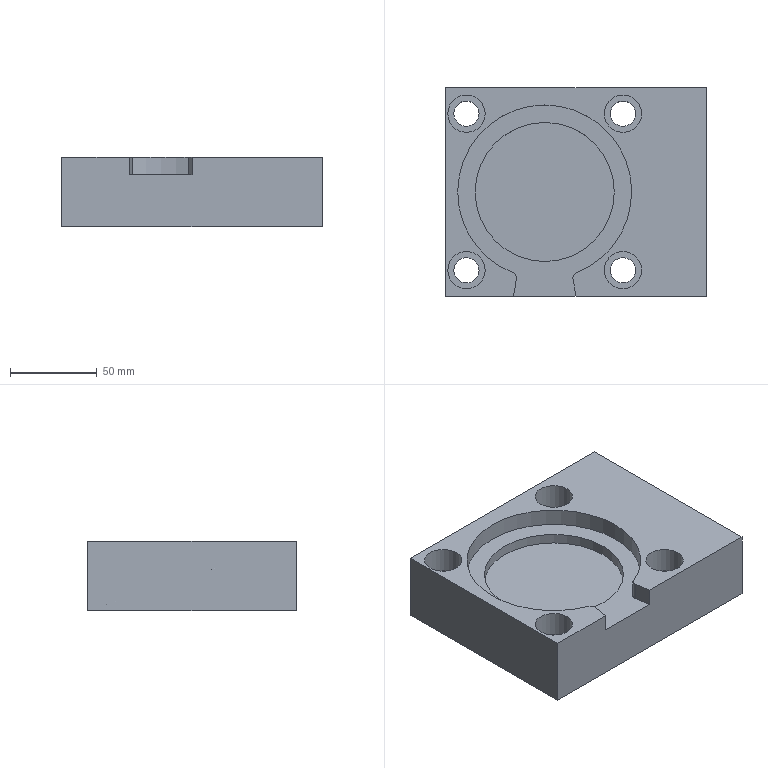Part | NX | 1 solid | 26 faces | box 150 x 120 x 40 mm | volume 569278 mm3 | plane 14 | cylinder 12 | commonest cylinder face diameters 14.5 x4 21.5 x4 6 x2 80 x1 100 x1
STEP:
#1=CARTESIAN_POINT('',(0.,-60.,-10.));
#2=VERTEX_POINT('',#1);
#3=CARTESIAN_POINT('',(-36.,-60.,-10.));
#4=VERTEX_POINT('',#3);
#5=CARTESIAN_POINT('',(0.,-60.,-10.));
#6=DIRECTION('',(-1.,0.,0.));
#7=VECTOR('',#6,1000.);
#8=LINE('',#5,#7);
#9=EDGE_CURVE('',#2,#4,#8,.T.);
#10=ORIENTED_EDGE('',*,*,#9,.T.);
#11=CARTESIAN_POINT('',(-36.,-60.,0.));
#12=VERTEX_POINT('',#11);
#13=CARTESIAN_POINT('',(-36.,-60.,-10.));
#14=DIRECTION('',(0.,0.,1.));
#15=VECTOR('',#14,1000.);
#16=LINE('',#13,#15);
#17=EDGE_CURVE('',#4,#12,#16,.T.);
#18=ORIENTED_EDGE('',*,*,#17,.T.);
#19=CARTESIAN_POINT('',(-75.,-60.,0.));
#20=VERTEX_POINT('',#19);
#21=CARTESIAN_POINT('',(-75.,-60.,0.));
#22=DIRECTION('',(1.,0.,0.));
#23=VECTOR('',#22,1000.);
#24=LINE('',#21,#23);
#25=EDGE_CURVE('',#20,#12,#24,.T.);
#26=ORIENTED_EDGE('',*,*,#25,.F.);
#27=CARTESIAN_POINT('',(-75.,-60.,-40.));
#28=VERTEX_POINT('',#27);
#29=CARTESIAN_POINT('',(-75.,-60.,-40.));
#30=DIRECTION('',(0.,0.,1.));
#31=VECTOR('',#30,1000.);
#32=LINE('',#29,#31);
#33=EDGE_CURVE('',#28,#20,#32,.T.);
#34=ORIENTED_EDGE('',*,*,#33,.F.);
#35=CARTESIAN_POINT('',(75.,-60.,-40.));
#36=VERTEX_POINT('',#35);
#37=CARTESIAN_POINT('',(-75.,-60.,-40.));
#38=DIRECTION('',(1.,0.,0.));
#39=VECTOR('',#38,1000.);
#40=LINE('',#37,#39);
#41=EDGE_CURVE('',#28,#36,#40,.T.);
#42=ORIENTED_EDGE('',*,*,#41,.T.);
#43=CARTESIAN_POINT('',(75.,-60.,0.));
#44=VERTEX_POINT('',#43);
#45=CARTESIAN_POINT('',(75.,-60.,-40.));
#46=DIRECTION('',(0.,0.,1.));
#47=VECTOR('',#46,1000.);
#48=LINE('',#45,#47);
#49=EDGE_CURVE('',#36,#44,#48,.T.);
#50=ORIENTED_EDGE('',*,*,#49,.T.);
#51=CARTESIAN_POINT('',(0.,-60.,0.));
#52=VERTEX_POINT('',#51);
#53=CARTESIAN_POINT('',(-75.,-60.,0.));
#54=DIRECTION('',(1.,0.,0.));
#55=VECTOR('',#54,1000.);
#56=LINE('',#53,#55);
#57=EDGE_CURVE('',#52,#44,#56,.T.);
#58=ORIENTED_EDGE('',*,*,#57,.F.);
#59=CARTESIAN_POINT('',(0.,-60.,-10.));
#60=DIRECTION('',(0.,0.,1.));
#61=VECTOR('',#60,1000.);
#62=LINE('',#59,#61);
#63=EDGE_CURVE('',#2,#52,#62,.T.);
#64=ORIENTED_EDGE('',*,*,#63,.F.);
#65=EDGE_LOOP('',(#10,#18,#26,#34,#42,#50,#58,#64));
#66=FACE_BOUND('',#65,.T.);
#67=CARTESIAN_POINT('',(-75.,-60.,-40.));
#68=DIRECTION('',(0.,-1.,0.));
#69=DIRECTION('',(0.,0.,-1.));
#70=AXIS2_PLACEMENT_3D('',#67,#68,#69);
#71=PLANE('',#70);
#72=ADVANCED_FACE('',(#66),#71,.T.);
#73=CARTESIAN_POINT('',(34.25,-45.,-40.));
#74=VERTEX_POINT('',#73);
#75=CARTESIAN_POINT('',(27.,-45.,-40.));
#76=DIRECTION('',(0.,0.,1.));
#77=DIRECTION('',(1.,0.,0.));
#78=AXIS2_PLACEMENT_3D('',#75,#76,#77);
#79=CIRCLE('',#78,7.25);
#80=EDGE_CURVE('',#74,#74,#79,.T.);
#81=ORIENTED_EDGE('',*,*,#80,.F.);
#82=EDGE_LOOP('',(#81));
#83=FACE_BOUND('',#82,.T.);
#84=CARTESIAN_POINT('',(34.25,-45.,-15.));
#85=VERTEX_POINT('',#84);
#86=CARTESIAN_POINT('',(27.,-45.,-15.));
#87=DIRECTION('',(0.,0.,1.));
#88=DIRECTION('',(1.,0.,0.));
#89=AXIS2_PLACEMENT_3D('',#86,#87,#88);
#90=CIRCLE('',#89,7.25);
#91=EDGE_CURVE('',#85,#85,#90,.F.);
#92=ORIENTED_EDGE('',*,*,#91,.F.);
#93=EDGE_LOOP('',(#92));
#94=FACE_BOUND('',#93,.T.);
#95=CARTESIAN_POINT('',(27.,-45.,-40.));
#96=DIRECTION('',(0.,0.,1.));
#97=DIRECTION('',(1.,0.,0.));
#98=AXIS2_PLACEMENT_3D('',#95,#96,#97);
#99=CYLINDRICAL_SURFACE('',#98,7.25);
#100=ADVANCED_FACE('',(#83,#94),#99,.F.);
#101=CARTESIAN_POINT('',(-55.75,45.,-40.));
#102=VERTEX_POINT('',#101);
#103=CARTESIAN_POINT('',(-63.,45.,-40.));
#104=DIRECTION('',(0.,0.,1.));
#105=DIRECTION('',(1.,0.,0.));
#106=AXIS2_PLACEMENT_3D('',#103,#104,#105);
#107=CIRCLE('',#106,7.25);
#108=EDGE_CURVE('',#102,#102,#107,.T.);
#109=ORIENTED_EDGE('',*,*,#108,.F.);
#110=EDGE_LOOP('',(#109));
#111=FACE_BOUND('',#110,.T.);
#112=CARTESIAN_POINT('',(-55.75,45.,-15.));
#113=VERTEX_POINT('',#112);
#114=CARTESIAN_POINT('',(-63.,45.,-15.));
#115=DIRECTION('',(0.,0.,1.));
#116=DIRECTION('',(1.,0.,0.));
#117=AXIS2_PLACEMENT_3D('',#114,#115,#116);
#118=CIRCLE('',#117,7.25);
#119=EDGE_CURVE('',#113,#113,#118,.F.);
#120=ORIENTED_EDGE('',*,*,#119,.F.);
#121=EDGE_LOOP('',(#120));
#122=FACE_BOUND('',#121,.T.);
#123=CARTESIAN_POINT('',(-63.,45.,-40.));
#124=DIRECTION('',(0.,0.,1.));
#125=DIRECTION('',(1.,0.,0.));
#126=AXIS2_PLACEMENT_3D('',#123,#124,#125);
#127=CYLINDRICAL_SURFACE('',#126,7.25);
#128=ADVANCED_FACE('',(#111,#122),#127,.F.);
#129=CARTESIAN_POINT('',(-55.75,-45.,-40.));
#130=VERTEX_POINT('',#129);
#131=CARTESIAN_POINT('',(-63.,-45.,-40.));
#132=DIRECTION('',(0.,0.,1.));
#133=DIRECTION('',(1.,0.,0.));
#134=AXIS2_PLACEMENT_3D('',#131,#132,#133);
#135=CIRCLE('',#134,7.25);
#136=EDGE_CURVE('',#130,#130,#135,.T.);
#137=ORIENTED_EDGE('',*,*,#136,.F.);
#138=EDGE_LOOP('',(#137));
#139=FACE_BOUND('',#138,.T.);
#140=CARTESIAN_POINT('',(-55.75,-45.,-15.));
#141=VERTEX_POINT('',#140);
#142=CARTESIAN_POINT('',(-63.,-45.,-15.));
#143=DIRECTION('',(0.,0.,1.));
#144=DIRECTION('',(1.,0.,0.));
#145=AXIS2_PLACEMENT_3D('',#142,#143,#144);
#146=CIRCLE('',#145,7.25);
#147=EDGE_CURVE('',#141,#141,#146,.F.);
#148=ORIENTED_EDGE('',*,*,#147,.F.);
#149=EDGE_LOOP('',(#148));
#150=FACE_BOUND('',#149,.T.);
#151=CARTESIAN_POINT('',(-63.,-45.,-40.));
#152=DIRECTION('',(0.,0.,1.));
#153=DIRECTION('',(1.,0.,0.));
#154=AXIS2_PLACEMENT_3D('',#151,#152,#153);
#155=CYLINDRICAL_SURFACE('',#154,7.25);
#156=ADVANCED_FACE('',(#139,#150),#155,.F.);
#157=CARTESIAN_POINT('',(34.25,45.,-40.));
#158=VERTEX_POINT('',#157);
#159=CARTESIAN_POINT('',(27.,45.,-40.));
#160=DIRECTION('',(0.,0.,1.));
#161=DIRECTION('',(1.,0.,0.));
#162=AXIS2_PLACEMENT_3D('',#159,#160,#161);
#163=CIRCLE('',#162,7.25);
#164=EDGE_CURVE('',#158,#158,#163,.T.);
#165=ORIENTED_EDGE('',*,*,#164,.F.);
#166=EDGE_LOOP('',(#165));
#167=FACE_BOUND('',#166,.T.);
#168=CARTESIAN_POINT('',(34.25,45.,-15.));
#169=VERTEX_POINT('',#168);
#170=CARTESIAN_POINT('',(27.,45.,-15.));
#171=DIRECTION('',(0.,0.,1.));
#172=DIRECTION('',(1.,0.,0.));
#173=AXIS2_PLACEMENT_3D('',#170,#171,#172);
#174=CIRCLE('',#173,7.25);
#175=EDGE_CURVE('',#169,#169,#174,.F.);
#176=ORIENTED_EDGE('',*,*,#175,.F.);
#177=EDGE_LOOP('',(#176));
#178=FACE_BOUND('',#177,.T.);
#179=CARTESIAN_POINT('',(27.,45.,-40.));
#180=DIRECTION('',(0.,0.,1.));
#181=DIRECTION('',(1.,0.,0.));
#182=AXIS2_PLACEMENT_3D('',#179,#180,#181);
#183=CYLINDRICAL_SURFACE('',#182,7.25);
#184=ADVANCED_FACE('',(#167,#178),#183,.F.);
#185=CARTESIAN_POINT('',(75.,60.,0.));
#186=VERTEX_POINT('',#185);
#187=CARTESIAN_POINT('',(75.,-60.,0.));
#188=DIRECTION('',(0.,1.,0.));
#189=VECTOR('',#188,1000.);
#190=LINE('',#187,#189);
#191=EDGE_CURVE('',#44,#186,#190,.T.);
#192=ORIENTED_EDGE('',*,*,#191,.F.);
#193=ORIENTED_EDGE('',*,*,#49,.F.);
#194=CARTESIAN_POINT('',(75.,60.,-40.));
#195=VERTEX_POINT('',#194);
#196=CARTESIAN_POINT('',(75.,-60.,-40.));
#197=DIRECTION('',(0.,1.,0.));
#198=VECTOR('',#197,1000.);
#199=LINE('',#196,#198);
#200=EDGE_CURVE('',#36,#195,#199,.T.);
#201=ORIENTED_EDGE('',*,*,#200,.T.);
#202=CARTESIAN_POINT('',(75.,60.,-40.));
#203=DIRECTION('',(0.,0.,1.));
#204=VECTOR('',#203,1000.);
#205=LINE('',#202,#204);
#206=EDGE_CURVE('',#195,#186,#205,.T.);
#207=ORIENTED_EDGE('',*,*,#206,.T.);
#208=EDGE_LOOP('',(#192,#193,#201,#207));
#209=FACE_BOUND('',#208,.T.);
#210=CARTESIAN_POINT('',(75.,-60.,-40.));
#211=DIRECTION('',(1.,0.,0.));
#212=DIRECTION('',(0.,1.,0.));
#213=AXIS2_PLACEMENT_3D('',#210,#211,#212);
#214=PLANE('',#213);
#215=ADVANCED_FACE('',(#209),#214,.T.);
#216=CARTESIAN_POINT('',(-75.,60.,0.));
#217=VERTEX_POINT('',#216);
#218=CARTESIAN_POINT('',(75.,60.,0.));
#219=DIRECTION('',(-1.,0.,0.));
#220=VECTOR('',#219,1000.);
#221=LINE('',#218,#220);
#222=EDGE_CURVE('',#186,#217,#221,.T.);
#223=ORIENTED_EDGE('',*,*,#222,.F.);
#224=ORIENTED_EDGE('',*,*,#206,.F.);
#225=CARTESIAN_POINT('',(-75.,60.,-40.));
#226=VERTEX_POINT('',#225);
#227=CARTESIAN_POINT('',(75.,60.,-40.));
#228=DIRECTION('',(-1.,0.,0.));
#229=VECTOR('',#228,1000.);
#230=LINE('',#227,#229);
#231=EDGE_CURVE('',#195,#226,#230,.T.);
#232=ORIENTED_EDGE('',*,*,#231,.T.);
#233=CARTESIAN_POINT('',(-75.,60.,-40.));
#234=DIRECTION('',(0.,0.,1.));
#235=VECTOR('',#234,1000.);
#236=LINE('',#233,#235);
#237=EDGE_CURVE('',#226,#217,#236,.T.);
#238=ORIENTED_EDGE('',*,*,#237,.T.);
#239=EDGE_LOOP('',(#223,#224,#232,#238));
#240=FACE_BOUND('',#239,.T.);
#241=CARTESIAN_POINT('',(75.,60.,-40.));
#242=DIRECTION('',(0.,1.,0.));
#243=DIRECTION('',(-1.,0.,0.));
#244=AXIS2_PLACEMENT_3D('',#241,#242,#243);
#245=PLANE('',#244);
#246=ADVANCED_FACE('',(#240),#245,.T.);
#247=CARTESIAN_POINT('',(-75.,60.,0.));
#248=DIRECTION('',(0.,-1.,0.));
#249=VECTOR('',#248,1000.);
#250=LINE('',#247,#249);
#251=EDGE_CURVE('',#217,#20,#250,.T.);
#252=ORIENTED_EDGE('',*,*,#251,.F.);
#253=ORIENTED_EDGE('',*,*,#237,.F.);
#254=CARTESIAN_POINT('',(-75.,60.,-40.));
#255=DIRECTION('',(0.,-1.,0.));
#256=VECTOR('',#255,1000.);
#257=LINE('',#254,#256);
#258=EDGE_CURVE('',#226,#28,#257,.T.);
#259=ORIENTED_EDGE('',*,*,#258,.T.);
#260=ORIENTED_EDGE('',*,*,#33,.T.);
#261=EDGE_LOOP('',(#252,#253,#259,#260));
#262=FACE_BOUND('',#261,.T.);
#263=CARTESIAN_POINT('',(-75.,60.,-40.));
#264=DIRECTION('',(-1.,0.,0.));
#265=DIRECTION('',(0.,-1.,0.));
#266=AXIS2_PLACEMENT_3D('',#263,#264,#265);
#267=PLANE('',#266);
#268=ADVANCED_FACE('',(#262),#267,.T.);
#269=ORIENTED_EDGE('',*,*,#41,.F.);
#270=ORIENTED_EDGE('',*,*,#258,.F.);
#271=ORIENTED_EDGE('',*,*,#231,.F.);
#272=ORIENTED_EDGE('',*,*,#200,.F.);
#273=EDGE_LOOP('',(#269,#270,#271,#272));
#274=FACE_BOUND('',#273,.T.);
#275=ORIENTED_EDGE('',*,*,#136,.T.);
#276=EDGE_LOOP('',(#275));
#277=FACE_BOUND('',#276,.T.);
#278=ORIENTED_EDGE('',*,*,#108,.T.);
#279=EDGE_LOOP('',(#278));
#280=FACE_BOUND('',#279,.T.);
#281=ORIENTED_EDGE('',*,*,#80,.T.);
#282=EDGE_LOOP('',(#281));
#283=FACE_BOUND('',#282,.T.);
#284=ORIENTED_EDGE('',*,*,#164,.T.);
#285=EDGE_LOOP('',(#284));
#286=FACE_BOUND('',#285,.T.);
#287=CARTESIAN_POINT('',(-63.,-45.,-40.));
#288=DIRECTION('',(0.,0.,1.));
#289=DIRECTION('',(1.,0.,0.));
#290=AXIS2_PLACEMENT_3D('',#287,#288,#289);
#291=PLANE('',#290);
#292=ADVANCED_FACE('',(#274,#277,#280,#283,#286),#291,.F.);
#293=CARTESIAN_POINT('',(37.75,-45.,0.));
#294=VERTEX_POINT('',#293);
#295=CARTESIAN_POINT('',(27.,-45.,0.));
#296=DIRECTION('',(0.,0.,1.));
#297=DIRECTION('',(1.,0.,0.));
#298=AXIS2_PLACEMENT_3D('',#295,#296,#297);
#299=CIRCLE('',#298,10.75);
#300=EDGE_CURVE('',#294,#294,#299,.T.);
#301=ORIENTED_EDGE('',*,*,#300,.F.);
#302=EDGE_LOOP('',(#301));
#303=FACE_BOUND('',#302,.T.);
#304=CARTESIAN_POINT('',(-52.25,45.,0.));
#305=VERTEX_POINT('',#304);
#306=CARTESIAN_POINT('',(-63.,45.,0.));
#307=DIRECTION('',(0.,0.,1.));
#308=DIRECTION('',(1.,0.,0.));
#309=AXIS2_PLACEMENT_3D('',#306,#307,#308);
#310=CIRCLE('',#309,10.75);
#311=EDGE_CURVE('',#305,#305,#310,.T.);
#312=ORIENTED_EDGE('',*,*,#311,.F.);
#313=EDGE_LOOP('',(#312));
#314=FACE_BOUND('',#313,.T.);
#315=CARTESIAN_POINT('',(-52.25,-45.,0.));
#316=VERTEX_POINT('',#315);
#317=CARTESIAN_POINT('',(-63.,-45.,0.));
#318=DIRECTION('',(0.,0.,1.));
#319=DIRECTION('',(1.,0.,0.));
#320=AXIS2_PLACEMENT_3D('',#317,#318,#319);
#321=CIRCLE('',#320,10.75);
#322=EDGE_CURVE('',#316,#316,#321,.T.);
#323=ORIENTED_EDGE('',*,*,#322,.F.);
#324=EDGE_LOOP('',(#323));
#325=FACE_BOUND('',#324,.T.);
#326=CARTESIAN_POINT('',(37.75,45.,0.));
#327=VERTEX_POINT('',#326);
#328=CARTESIAN_POINT('',(27.,45.,0.));
#329=DIRECTION('',(0.,0.,1.));
#330=DIRECTION('',(1.,0.,0.));
#331=AXIS2_PLACEMENT_3D('',#328,#329,#330);
#332=CIRCLE('',#331,10.75);
#333=EDGE_CURVE('',#327,#327,#332,.T.);
#334=ORIENTED_EDGE('',*,*,#333,.F.);
#335=EDGE_LOOP('',(#334));
#336=FACE_BOUND('',#335,.T.);
#337=CARTESIAN_POINT('',(-36.093,-46.612,0.));
#338=VERTEX_POINT('',#337);
#339=CARTESIAN_POINT('',(0.09309,-46.612,0.));
#340=VERTEX_POINT('',#339);
#341=CARTESIAN_POINT('',(-18.,0.,0.));
#342=DIRECTION('',(0.,0.,-1.));
#343=DIRECTION('',(1.,0.,0.));
#344=AXIS2_PLACEMENT_3D('',#341,#342,#343);
#345=CIRCLE('',#344,50.);
#346=EDGE_CURVE('',#338,#340,#345,.T.);
#347=ORIENTED_EDGE('',*,*,#346,.T.);
#348=CARTESIAN_POINT('',(-1.776,-49.929,0.));
#349=VERTEX_POINT('',#348);
#350=CARTESIAN_POINT('',(1.179,-49.408,0.));
#351=DIRECTION('',(0.,0.,1.));
#352=DIRECTION('',(1.,0.,0.));
#353=AXIS2_PLACEMENT_3D('',#350,#351,#352);
#354=CIRCLE('',#353,3.);
#355=EDGE_CURVE('',#340,#349,#354,.T.);
#356=ORIENTED_EDGE('',*,*,#355,.T.);
#357=CARTESIAN_POINT('',(-2.214,-47.443,0.));
#358=DIRECTION('',(0.1736,-0.9848,0.));
#359=VECTOR('',#358,1000.);
#360=LINE('',#357,#359);
#361=EDGE_CURVE('',#349,#52,#360,.T.);
#362=ORIENTED_EDGE('',*,*,#361,.T.);
#363=ORIENTED_EDGE('',*,*,#57,.T.);
#364=ORIENTED_EDGE('',*,*,#191,.T.);
#365=ORIENTED_EDGE('',*,*,#222,.T.);
#366=ORIENTED_EDGE('',*,*,#251,.T.);
#367=ORIENTED_EDGE('',*,*,#25,.T.);
#368=CARTESIAN_POINT('',(-34.224,-49.929,0.));
#369=VERTEX_POINT('',#368);
#370=CARTESIAN_POINT('',(-36.,-60.,0.));
#371=DIRECTION('',(0.1736,0.9848,0.));
#372=VECTOR('',#371,1000.);
#373=LINE('',#370,#372);
#374=EDGE_CURVE('',#12,#369,#373,.T.);
#375=ORIENTED_EDGE('',*,*,#374,.T.);
#376=CARTESIAN_POINT('',(-37.179,-49.408,0.));
#377=DIRECTION('',(0.,0.,1.));
#378=DIRECTION('',(1.,0.,0.));
#379=AXIS2_PLACEMENT_3D('',#376,#377,#378);
#380=CIRCLE('',#379,3.);
#381=EDGE_CURVE('',#369,#338,#380,.T.);
#382=ORIENTED_EDGE('',*,*,#381,.T.);
#383=EDGE_LOOP('',(#347,#356,#362,#363,#364,#365,#366,#367,#375,#382));
#384=FACE_BOUND('',#383,.T.);
#385=CARTESIAN_POINT('',(-63.,-45.,0.));
#386=DIRECTION('',(0.,0.,1.));
#387=DIRECTION('',(1.,0.,0.));
#388=AXIS2_PLACEMENT_3D('',#385,#386,#387);
#389=PLANE('',#388);
#390=ADVANCED_FACE('',(#303,#314,#325,#336,#384),#389,.T.);
#391=CARTESIAN_POINT('',(37.75,45.,-15.));
#392=VERTEX_POINT('',#391);
#393=CARTESIAN_POINT('',(27.,45.,-15.));
#394=DIRECTION('',(0.,0.,1.));
#395=DIRECTION('',(1.,0.,0.));
#396=AXIS2_PLACEMENT_3D('',#393,#394,#395);
#397=CIRCLE('',#396,10.75);
#398=EDGE_CURVE('',#392,#392,#397,.F.);
#399=ORIENTED_EDGE('',*,*,#398,.F.);
#400=EDGE_LOOP('',(#399));
#401=FACE_BOUND('',#400,.T.);
#402=ORIENTED_EDGE('',*,*,#175,.T.);
#403=EDGE_LOOP('',(#402));
#404=FACE_BOUND('',#403,.T.);
#405=CARTESIAN_POINT('',(27.,45.,-15.));
#406=DIRECTION('',(0.,0.,1.));
#407=DIRECTION('',(1.,0.,0.));
#408=AXIS2_PLACEMENT_3D('',#405,#406,#407);
#409=PLANE('',#408);
#410=ADVANCED_FACE('',(#401,#404),#409,.T.);
#411=ORIENTED_EDGE('',*,*,#398,.T.);
#412=EDGE_LOOP('',(#411));
#413=FACE_BOUND('',#412,.T.);
#414=ORIENTED_EDGE('',*,*,#333,.T.);
#415=EDGE_LOOP('',(#414));
#416=FACE_BOUND('',#415,.T.);
#417=CARTESIAN_POINT('',(27.,45.,-15.));
#418=DIRECTION('',(0.,0.,1.));
#419=DIRECTION('',(1.,0.,0.));
#420=AXIS2_PLACEMENT_3D('',#417,#418,#419);
#421=CYLINDRICAL_SURFACE('',#420,10.75);
#422=ADVANCED_FACE('',(#413,#416),#421,.F.);
#423=CARTESIAN_POINT('',(-52.25,-45.,-15.));
#424=VERTEX_POINT('',#423);
#425=CARTESIAN_POINT('',(-63.,-45.,-15.));
#426=DIRECTION('',(0.,0.,1.));
#427=DIRECTION('',(1.,0.,0.));
#428=AXIS2_PLACEMENT_3D('',#425,#426,#427);
#429=CIRCLE('',#428,10.75);
#430=EDGE_CURVE('',#424,#424,#429,.F.);
#431=ORIENTED_EDGE('',*,*,#430,.F.);
#432=EDGE_LOOP('',(#431));
#433=FACE_BOUND('',#432,.T.);
#434=ORIENTED_EDGE('',*,*,#147,.T.);
#435=EDGE_LOOP('',(#434));
#436=FACE_BOUND('',#435,.T.);
#437=CARTESIAN_POINT('',(-63.,-45.,-15.));
#438=DIRECTION('',(0.,0.,1.));
#439=DIRECTION('',(1.,0.,0.));
#440=AXIS2_PLACEMENT_3D('',#437,#438,#439);
#441=PLANE('',#440);
#442=ADVANCED_FACE('',(#433,#436),#441,.T.);
#443=ORIENTED_EDGE('',*,*,#430,.T.);
#444=EDGE_LOOP('',(#443));
#445=FACE_BOUND('',#444,.T.);
#446=ORIENTED_EDGE('',*,*,#322,.T.);
#447=EDGE_LOOP('',(#446));
#448=FACE_BOUND('',#447,.T.);
#449=CARTESIAN_POINT('',(-63.,-45.,-15.));
#450=DIRECTION('',(0.,0.,1.));
#451=DIRECTION('',(1.,0.,0.));
#452=AXIS2_PLACEMENT_3D('',#449,#450,#451);
#453=CYLINDRICAL_SURFACE('',#452,10.75);
#454=ADVANCED_FACE('',(#445,#448),#453,.F.);
#455=CARTESIAN_POINT('',(-52.25,45.,-15.));
#456=VERTEX_POINT('',#455);
#457=CARTESIAN_POINT('',(-63.,45.,-15.));
#458=DIRECTION('',(0.,0.,1.));
#459=DIRECTION('',(1.,0.,0.));
#460=AXIS2_PLACEMENT_3D('',#457,#458,#459);
#461=CIRCLE('',#460,10.75);
#462=EDGE_CURVE('',#456,#456,#461,.F.);
#463=ORIENTED_EDGE('',*,*,#462,.F.);
#464=EDGE_LOOP('',(#463));
#465=FACE_BOUND('',#464,.T.);
#466=ORIENTED_EDGE('',*,*,#119,.T.);
#467=EDGE_LOOP('',(#466));
#468=FACE_BOUND('',#467,.T.);
#469=CARTESIAN_POINT('',(-63.,45.,-15.));
#470=DIRECTION('',(0.,0.,1.));
#471=DIRECTION('',(1.,0.,0.));
#472=AXIS2_PLACEMENT_3D('',#469,#470,#471);
#473=PLANE('',#472);
#474=ADVANCED_FACE('',(#465,#468),#473,.T.);
#475=ORIENTED_EDGE('',*,*,#462,.T.);
#476=EDGE_LOOP('',(#475));
#477=FACE_BOUND('',#476,.T.);
#478=ORIENTED_EDGE('',*,*,#311,.T.);
#479=EDGE_LOOP('',(#478));
#480=FACE_BOUND('',#479,.T.);
#481=CARTESIAN_POINT('',(-63.,45.,-15.));
#482=DIRECTION('',(0.,0.,1.));
#483=DIRECTION('',(1.,0.,0.));
#484=AXIS2_PLACEMENT_3D('',#481,#482,#483);
#485=CYLINDRICAL_SURFACE('',#484,10.75);
#486=ADVANCED_FACE('',(#477,#480),#485,.F.);
#487=CARTESIAN_POINT('',(37.75,-45.,-15.));
#488=VERTEX_POINT('',#487);
#489=CARTESIAN_POINT('',(27.,-45.,-15.));
#490=DIRECTION('',(0.,0.,1.));
#491=DIRECTION('',(1.,0.,0.));
#492=AXIS2_PLACEMENT_3D('',#489,#490,#491);
#493=CIRCLE('',#492,10.75);
#494=EDGE_CURVE('',#488,#488,#493,.F.);
#495=ORIENTED_EDGE('',*,*,#494,.F.);
#496=EDGE_LOOP('',(#495));
#497=FACE_BOUND('',#496,.T.);
#498=ORIENTED_EDGE('',*,*,#91,.T.);
#499=EDGE_LOOP('',(#498));
#500=FACE_BOUND('',#499,.T.);
#501=CARTESIAN_POINT('',(27.,-45.,-15.));
#502=DIRECTION('',(0.,0.,1.));
#503=DIRECTION('',(1.,0.,0.));
#504=AXIS2_PLACEMENT_3D('',#501,#502,#503);
#505=PLANE('',#504);
#506=ADVANCED_FACE('',(#497,#500),#505,.T.);
#507=ORIENTED_EDGE('',*,*,#494,.T.);
#508=EDGE_LOOP('',(#507));
#509=FACE_BOUND('',#508,.T.);
#510=ORIENTED_EDGE('',*,*,#300,.T.);
#511=EDGE_LOOP('',(#510));
#512=FACE_BOUND('',#511,.T.);
#513=CARTESIAN_POINT('',(27.,-45.,-15.));
#514=DIRECTION('',(0.,0.,1.));
#515=DIRECTION('',(1.,0.,0.));
#516=AXIS2_PLACEMENT_3D('',#513,#514,#515);
#517=CYLINDRICAL_SURFACE('',#516,10.75);
#518=ADVANCED_FACE('',(#509,#512),#517,.F.);
#519=ORIENTED_EDGE('',*,*,#9,.F.);
#520=CARTESIAN_POINT('',(-1.776,-49.929,-10.));
#521=VERTEX_POINT('',#520);
#522=CARTESIAN_POINT('',(-2.214,-47.443,-10.));
#523=DIRECTION('',(0.1736,-0.9848,0.));
#524=VECTOR('',#523,1000.);
#525=LINE('',#522,#524);
#526=EDGE_CURVE('',#2,#521,#525,.F.);
#527=ORIENTED_EDGE('',*,*,#526,.T.);
#528=CARTESIAN_POINT('',(0.09309,-46.612,-10.));
#529=VERTEX_POINT('',#528);
#530=CARTESIAN_POINT('',(1.179,-49.408,-10.));
#531=DIRECTION('',(0.,0.,-1.));
#532=DIRECTION('',(-1.,0.,0.));
#533=AXIS2_PLACEMENT_3D('',#530,#531,#532);
#534=CIRCLE('',#533,3.);
#535=EDGE_CURVE('',#521,#529,#534,.T.);
#536=ORIENTED_EDGE('',*,*,#535,.T.);
#537=CARTESIAN_POINT('',(-36.093,-46.612,-10.));
#538=VERTEX_POINT('',#537);
#539=CARTESIAN_POINT('',(-18.,0.,-10.));
#540=DIRECTION('',(0.,0.,-1.));
#541=DIRECTION('',(1.,0.,0.));
#542=AXIS2_PLACEMENT_3D('',#539,#540,#541);
#543=CIRCLE('',#542,50.);
#544=EDGE_CURVE('',#529,#538,#543,.F.);
#545=ORIENTED_EDGE('',*,*,#544,.T.);
#546=CARTESIAN_POINT('',(-34.224,-49.929,-10.));
#547=VERTEX_POINT('',#546);
#548=CARTESIAN_POINT('',(-37.179,-49.408,-10.));
#549=DIRECTION('',(0.,0.,-1.));
#550=DIRECTION('',(-1.,0.,0.));
#551=AXIS2_PLACEMENT_3D('',#548,#549,#550);
#552=CIRCLE('',#551,3.);
#553=EDGE_CURVE('',#538,#547,#552,.T.);
#554=ORIENTED_EDGE('',*,*,#553,.T.);
#555=CARTESIAN_POINT('',(-36.,-60.,-10.));
#556=DIRECTION('',(0.1736,0.9848,0.));
#557=VECTOR('',#556,1000.);
#558=LINE('',#555,#557);
#559=EDGE_CURVE('',#547,#4,#558,.F.);
#560=ORIENTED_EDGE('',*,*,#559,.T.);
#561=EDGE_LOOP('',(#519,#527,#536,#545,#554,#560));
#562=FACE_BOUND('',#561,.T.);
#563=CARTESIAN_POINT('',(-58.,0.,-10.));
#564=VERTEX_POINT('',#563);
#565=CARTESIAN_POINT('',(-18.,0.,-10.));
#566=DIRECTION('',(0.,0.,-1.));
#567=DIRECTION('',(-1.,0.,0.));
#568=AXIS2_PLACEMENT_3D('',#565,#566,#567);
#569=CIRCLE('',#568,40.);
#570=EDGE_CURVE('',#564,#564,#569,.F.);
#571=ORIENTED_EDGE('',*,*,#570,.F.);
#572=EDGE_LOOP('',(#571));
#573=FACE_BOUND('',#572,.T.);
#574=CARTESIAN_POINT('',(-18.,0.,-10.));
#575=DIRECTION('',(0.,0.,-1.));
#576=DIRECTION('',(-1.,0.,0.));
#577=AXIS2_PLACEMENT_3D('',#574,#575,#576);
#578=PLANE('',#577);
#579=ADVANCED_FACE('',(#562,#573),#578,.F.);
#580=ORIENTED_EDGE('',*,*,#559,.F.);
#581=CARTESIAN_POINT('',(-34.224,-49.929,-10.));
#582=DIRECTION('',(0.,0.,1.));
#583=VECTOR('',#582,1000.);
#584=LINE('',#581,#583);
#585=EDGE_CURVE('',#547,#369,#584,.T.);
#586=ORIENTED_EDGE('',*,*,#585,.T.);
#587=ORIENTED_EDGE('',*,*,#374,.F.);
#588=ORIENTED_EDGE('',*,*,#17,.F.);
#589=EDGE_LOOP('',(#580,#586,#587,#588));
#590=FACE_BOUND('',#589,.T.);
#591=CARTESIAN_POINT('',(-36.,-60.,-10.));
#592=DIRECTION('',(0.9848,-0.1736,0.));
#593=DIRECTION('',(0.1736,0.9848,0.));
#594=AXIS2_PLACEMENT_3D('',#591,#592,#593);
#595=PLANE('',#594);
#596=ADVANCED_FACE('',(#590),#595,.T.);
#597=ORIENTED_EDGE('',*,*,#544,.F.);
#598=CARTESIAN_POINT('',(0.09309,-46.612,-10.));
#599=DIRECTION('',(0.,0.,1.));
#600=VECTOR('',#599,1000.);
#601=LINE('',#598,#600);
#602=EDGE_CURVE('',#529,#340,#601,.T.);
#603=ORIENTED_EDGE('',*,*,#602,.T.);
#604=ORIENTED_EDGE('',*,*,#346,.F.);
#605=CARTESIAN_POINT('',(-36.093,-46.612,-10.));
#606=DIRECTION('',(0.,0.,1.));
#607=VECTOR('',#606,1000.);
#608=LINE('',#605,#607);
#609=EDGE_CURVE('',#338,#538,#608,.F.);
#610=ORIENTED_EDGE('',*,*,#609,.T.);
#611=EDGE_LOOP('',(#597,#603,#604,#610));
#612=FACE_BOUND('',#611,.T.);
#613=CARTESIAN_POINT('',(-18.,0.,-10.));
#614=DIRECTION('',(0.,0.,1.));
#615=DIRECTION('',(1.,0.,0.));
#616=AXIS2_PLACEMENT_3D('',#613,#614,#615);
#617=CYLINDRICAL_SURFACE('',#616,50.);
#618=ADVANCED_FACE('',(#612),#617,.F.);
#619=ORIENTED_EDGE('',*,*,#361,.F.);
#620=CARTESIAN_POINT('',(-1.776,-49.929,-10.));
#621=DIRECTION('',(0.,0.,1.));
#622=VECTOR('',#621,1000.);
#623=LINE('',#620,#622);
#624=EDGE_CURVE('',#349,#521,#623,.F.);
#625=ORIENTED_EDGE('',*,*,#624,.T.);
#626=ORIENTED_EDGE('',*,*,#526,.F.);
#627=ORIENTED_EDGE('',*,*,#63,.T.);
#628=EDGE_LOOP('',(#619,#625,#626,#627));
#629=FACE_BOUND('',#628,.T.);
#630=CARTESIAN_POINT('',(-2.214,-47.443,-10.));
#631=DIRECTION('',(-0.9848,-0.1736,0.));
#632=DIRECTION('',(0.1736,-0.9848,0.));
#633=AXIS2_PLACEMENT_3D('',#630,#631,#632);
#634=PLANE('',#633);
#635=ADVANCED_FACE('',(#629),#634,.T.);
#636=CARTESIAN_POINT('',(22.,0.,-16.));
#637=VERTEX_POINT('',#636);
#638=CARTESIAN_POINT('',(-18.,0.,-16.));
#639=DIRECTION('',(0.,0.,1.));
#640=DIRECTION('',(1.,0.,0.));
#641=AXIS2_PLACEMENT_3D('',#638,#639,#640);
#642=CIRCLE('',#641,40.);
#643=EDGE_CURVE('',#637,#637,#642,.F.);
#644=ORIENTED_EDGE('',*,*,#643,.F.);
#645=EDGE_LOOP('',(#644));
#646=FACE_BOUND('',#645,.T.);
#647=CARTESIAN_POINT('',(-18.,0.,-16.));
#648=DIRECTION('',(0.,0.,1.));
#649=DIRECTION('',(1.,0.,0.));
#650=AXIS2_PLACEMENT_3D('',#647,#648,#649);
#651=PLANE('',#650);
#652=ADVANCED_FACE('',(#646),#651,.T.);
#653=ORIENTED_EDGE('',*,*,#570,.T.);
#654=EDGE_LOOP('',(#653));
#655=FACE_BOUND('',#654,.T.);
#656=ORIENTED_EDGE('',*,*,#643,.T.);
#657=EDGE_LOOP('',(#656));
#658=FACE_BOUND('',#657,.T.);
#659=CARTESIAN_POINT('',(-18.,0.,-16.));
#660=DIRECTION('',(0.,0.,1.));
#661=DIRECTION('',(1.,0.,0.));
#662=AXIS2_PLACEMENT_3D('',#659,#660,#661);
#663=CYLINDRICAL_SURFACE('',#662,40.);
#664=ADVANCED_FACE('',(#655,#658),#663,.F.);
#665=ORIENTED_EDGE('',*,*,#355,.F.);
#666=ORIENTED_EDGE('',*,*,#602,.F.);
#667=ORIENTED_EDGE('',*,*,#535,.F.);
#668=ORIENTED_EDGE('',*,*,#624,.F.);
#669=EDGE_LOOP('',(#665,#666,#667,#668));
#670=FACE_BOUND('',#669,.T.);
#671=CARTESIAN_POINT('',(1.179,-49.408,-10.));
#672=DIRECTION('',(0.,0.,1.));
#673=DIRECTION('',(1.,0.,0.));
#674=AXIS2_PLACEMENT_3D('',#671,#672,#673);
#675=CYLINDRICAL_SURFACE('',#674,3.);
#676=ADVANCED_FACE('',(#670),#675,.T.);
#677=ORIENTED_EDGE('',*,*,#381,.F.);
#678=ORIENTED_EDGE('',*,*,#585,.F.);
#679=ORIENTED_EDGE('',*,*,#553,.F.);
#680=ORIENTED_EDGE('',*,*,#609,.F.);
#681=EDGE_LOOP('',(#677,#678,#679,#680));
#682=FACE_BOUND('',#681,.T.);
#683=CARTESIAN_POINT('',(-37.179,-49.408,-10.));
#684=DIRECTION('',(0.,0.,1.));
#685=DIRECTION('',(1.,0.,0.));
#686=AXIS2_PLACEMENT_3D('',#683,#684,#685);
#687=CYLINDRICAL_SURFACE('',#686,3.);
#688=ADVANCED_FACE('',(#682),#687,.T.);
#689=CLOSED_SHELL('',(#72,#100,#128,#156,#184,#215,#246,#268,#292,#390,#410,#422,#442,#454,#474,#486,#506,#518,#579,#596,#618,#635,#652,#664,#676,#688));
#690=MANIFOLD_SOLID_BREP('',#689);
#691=(LENGTH_UNIT()NAMED_UNIT(*)SI_UNIT(.MILLI.,.METRE.));
#692=UNCERTAINTY_MEASURE_WITH_UNIT(LENGTH_MEASURE(0.00001),#691,'','');
#693=(NAMED_UNIT(*)PLANE_ANGLE_UNIT()SI_UNIT($,.RADIAN.));
#694=(NAMED_UNIT(*)SI_UNIT($,.STERADIAN.)SOLID_ANGLE_UNIT());
#695=(GEOMETRIC_REPRESENTATION_CONTEXT(3)GLOBAL_UNCERTAINTY_ASSIGNED_CONTEXT((#692))GLOBAL_UNIT_ASSIGNED_CONTEXT((#691,#693,#694))REPRESENTATION_CONTEXT('',''));
#696=ADVANCED_BREP_SHAPE_REPRESENTATION('',(#690),#695);